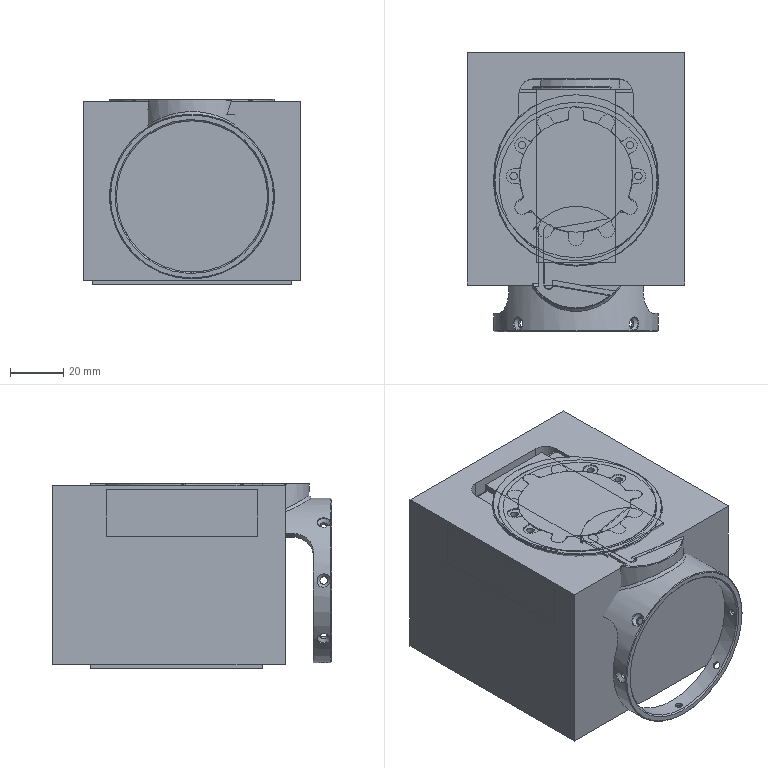NC program | NX | posted with a generic post | part box 82 x 105.2 x 70 mm
Lines 1 to 1140 of 2964:
N10 G17 G21 G94 G90
(外形动态铣_2 , TOOL : 粗刀D10)
N12 T15 M6
N14 G53
N16 G17 G0 G90 X-52.043 Y-12.093 B0. C0. S8500 M3
N18 G43 Z10. H15
N20 G94 G1 Z-1.42 F4500.
N22 Z-2.42
N24 X-50.413 Y-11.807
N26 G3 X-50.062 Y-11.562 R0.505
N28 X-49.643 Y-10.589 R3.413
N30 X-49.24 Y-8.159 R13.674
N32 X-49.052 Y-4.148 R57.416
N34 X-48.999 Y6.539 R617.695
N36 G1 X-48.995 Y30.289
N38 G2 X-48.67 Y32.126 R5.442
N40 X-47.193 Y34.11 R4.969
N42 X-44.793 Y35.433 R7.843
N44 X-41.628 Y36.142 R15.116
N46 X-37.264 Y36.43 R45.199
N48 X-28.39 Y36.499 R363.791
N50 G1 X42.61 Y36.498
N52 G2 X44.458 Y36.233 R5.973
N54 X46.495 Y34.832 R4.826
N56 X47.87 Y32.468 R7.551
N58 X48.602 Y29.434 R14.17
N60 X48.909 Y25.448 R38.306
N62 X48.997 Y17.949 R240.76
N64 G1 X48.995 Y-30.301
N66 G2 X48.668 Y-32.138 R5.474
N68 X47.277 Y-34.034 R4.92
N70 X45.018 Y-35.348 R7.552
N72 X41.866 Y-36.11 R14.168
N74 X37.629 Y-36.419 R41.423
N76 X29.755 Y-36.498 R283.099
N78 G1 X-42.745 Y-36.495
N80 G2 X-44.585 Y-36.186 R5.514
N82 X-46.579 Y-34.723 R4.919
N84 X-47.873 Y-32.444 R7.748
N86 X-48.621 Y-29.283 R14.522
N88 X-48.909 Y-25.42 R38.94
N90 X-48.998 Y-18.171 R233.446
N92 X-48.992 Y-14.546 R296.157
N94 X-48.757 Y-12.183 R24.037
N96 G3 X-48.103 Y-4.487 R64.834
N98 X-48.005 Y2.426 R246.922
N100 X-48. Y10.665 R1000.
N102 G1 X-47.999 Y27.917
N104 G2 X-46.344 Y32.109 R5.886
N106 X-43.67 Y33.95 R8.334
N108 X-40.441 Y34.904 R14.019
N110 X-36.342 Y35.342 R32.642
N112 X-30.219 Y35.486 R134.565
N114 X-24.094 Y35.499 R1000.
N116 G1 X40.416 Y35.498
N118 G2 X44.609 Y33.845 R5.88
N120 X46.45 Y31.17 R8.332
N122 X47.404 Y27.94 R14.057
N124 X47.842 Y23.841 R32.645
N126 X47.986 Y17.719 R134.554
N128 X47.999 Y11.594 R1000.
N130 G1 X47.998 Y-27.906
N132 G2 X46.348 Y-32.101 R5.882
N134 X43.671 Y-33.947 R8.336
N136 X40.442 Y-34.903 R14.049
N138 X36.343 Y-35.342 R32.586
N140 X30.22 Y-35.486 R134.246
N142 X23.97 Y-35.499 R1000.
N144 G1 X-40.416 Y-35.498
N146 G2 X-44.608 Y-33.841 R5.895
N148 X-46.447 Y-31.171 R8.316
N150 X-47.403 Y-27.941 R14.016
N152 X-47.842 Y-23.843 R32.589
N154 X-47.978 Y-16.22 R133.037
N156 X-47.763 Y-12.978 R44.65
N158 G3 X-47.291 Y-7.633 R159.7
N160 X-47.032 Y0.199 R149.4
N162 X-46.999 Y12.038 R1000.
N164 G1 X-46.996 Y25.913
N166 G2 X-46.54 Y28.484 R7.422
N168 X-44.24 Y31.56 R7.209
N170 X-41.152 Y33.205 R10.519
N172 X-37.375 Y34.05 R19.181
N174 X-32.64 Y34.399 R49.593
N176 X-25.141 Y34.496 R237.63
N178 G1 X38.359
N180 G2 X41.282 Y33.917 R7.449
N182 X44.32 Y31.392 R7.377
N184 X45.835 Y28.253 R11.074
N186 X46.602 Y24.458 R20.664
N188 X46.923 Y19.344 R57.679
N190 X46.998 Y9.97 R373.189
N192 G1 X46.995 Y-25.905
N194 G2 X46.446 Y-28.708 R7.345
N196 X44.241 Y-31.556 R7.239
N198 X41.153 Y-33.203 R10.504
N200 X37.378 Y-34.049 R19.152
N202 X32.643 Y-34.399 R49.518
N204 X25.144 Y-34.497 R234.014
N206 G1 X-38.356 Y-34.495
N208 G2 X-41.279 Y-33.916 R7.474
N210 X-44.32 Y-31.388 R7.386
N212 X-45.805 Y-28.35 R10.943
N214 X-46.603 Y-24.437 R20.53
N216 X-46.917 Y-19.573 R56.206
N218 X-46.738 Y-13.329 R55.96
N220 G3 X-46.333 Y-8.017 R338.621
N222 X-46.036 Y0.826 R173.15
N224 X-45.997 Y7.041 R606.66
N226 G1 X-45.995 Y23.915
N228 G2 X-45.649 Y26.509 R9.755
N230 X-43.262 Y30.146 R7.592
N232 X-40.135 Y31.967 R10.648
N234 X-36.264 Y32.943 R18.429
N236 X-31.285 Y33.372 R46.14
N238 X-24.161 Y33.493 R207.022
N240 G1 X35.839 Y33.498
N242 G2 X37.958 Y33.376 R13.815
N244 X42.673 Y30.725 R7.611
N246 X44.523 Y27.479 R10.701
N248 X45.466 Y23.6 R18.976
N250 X45.879 Y18.619 R48.048
N252 X45.994 Y11.12 R216.833
N254 G1 Y-23.88
N256 G2 X45.656 Y-26.474 R9.709
N258 X43.217 Y-30.181 R7.682
N260 X39.942 Y-32.038 R10.821
N262 X36.181 Y-32.955 R18.916
N264 X31.451 Y-33.364 R44.813
N266 X24.453 Y-33.492 R189.178
N268 G1 X19.453 Y-33.498
N270 X-36.422 Y-33.494
N272 G2 X-39.016 Y-33.145 R9.759
N274 X-42.642 Y-30.762 R7.606
N276 X-44.465 Y-27.636 R10.626
N278 X-45.461 Y-23.642 R18.622
N280 X-45.836 Y-16.285 R42.637
N282 X-45.592 Y-11.792 R107.085
N284 G3 X-45.034 Y1.823 R203.464
N286 X-44.999 Y14.288 R986.967
N288 G2 X-44.991 Y22.288 R944.802
N290 X-44.699 Y24.766 R11.344
N292 X-41.906 Y29.128 R8.152
N294 X-38.51 Y31.005 R11.434
N296 X-34.501 Y31.955 R20.428
N298 X-29.52 Y32.368 R50.119
N300 X-22.022 Y32.493 R213.614
N302 G1 X34.228 Y32.497
N304 G2 X36.595 Y32.333 R14.646
N306 X41.655 Y29.368 R8.135
N308 X43.47 Y26.094 R11.388
N310 X44.44 Y22.091 R20.004
N312 X44.865 Y17.111 R48.962
N314 X44.99 Y10.237 R197.067
N316 G1 X44.998 Y4.112
N318 X44.994 Y-22.013
N320 G2 X44.732 Y-24.619 R12.373
N322 X42.034 Y-29.016 R8.101
N324 X38.69 Y-30.935 R11.157
N326 X34.817 Y-31.908 R19.575
N328 X29.84 Y-32.355 R46.557
N330 X23.842 Y-32.483 R158.331
N332 X16.592 Y-32.498 R1000.
N334 G1 X-34.533 Y-32.494
N336 G2 X-37.018 Y-32.254 R12.688
N338 X-41.625 Y-29.404 R8.134
N340 X-43.503 Y-26.011 R11.403
N342 X-44.484 Y-21.753 R20.375
N344 X-44.75 Y-16.265 R38.136
N346 X-44.512 Y-10.895 R123.265
N348 G3 X-44.033 Y2.571 R242.716
N350 X-43.999 Y14.912 R1000.
N352 G2 X-43.988 Y20.662 R450.284
N354 X-43.674 Y23.389 R12.708
N356 X-40.889 Y27.883 R8.511
N358 X-37.744 Y29.75 R11.416
N360 X-33.893 Y30.804 R18.865
N362 X-29.297 Y31.296 R41.022
N364 X-22.925 Y31.476 R130.557
N366 X-16.175 Y31.497 R711.258
N368 G1 X-1.22 Y31.499
N370 G2 X0.49 Y31.58 R8.636
N372 G3 X8.042 Y31.498 R299.667
N374 G1 X32.791 Y31.493
N376 G2 X35.281 Y31.298 R15.428
N378 X40.466 Y28.285 R8.529
N380 X42.384 Y24.896 R11.816
N382 X43.403 Y20.778 R20.455
N384 X43.863 Y15.425 R50.095
N386 X43.992 Y7.927 R211.024
N388 G1 X43.998 Y-19.573
N390 G2 X43.885 Y-22.194 R22.421
N392 X42.721 Y-25.729 R8.758
N394 X40.142 Y-28.457 R8.995
N396 X36.654 Y-30.141 R12.821
N398 X32.376 Y-31.027 R23.489
N400 X26.891 Y-31.401 R60.265
N402 X17.642 Y-31.496 R327.657
N404 G1 X-32.733 Y-31.494
N406 G2 X-35.347 Y-31.288 R15.502
N408 X-40.677 Y-28.019 R8.552
N410 X-42.485 Y-24.611 R12.022
N412 X-43.427 Y-20.345 R19.892
N414 X-43.644 Y-15.228 R39.456
N416 X-43.495 Y-10.981 R124.985
N418 G3 X-43.013 Y5.432 R315.824
N420 X-42.997 Y14.911 R1000.
N422 G2 X-42.981 Y19.286 R191.99
N424 X-42.638 Y22.135 R13.374
N426 X-39.405 Y27.061 R8.879
N428 X-35.871 Y28.942 R12.502
N430 X-31.862 Y29.894 R21.869
N432 X-26.635 Y30.351 R50.776
N434 X-20.011 Y30.485 R179.698
N436 X-14.761 Y30.497 R672.427
N438 G1 X-4.209
N440 G3 X-3.912 Y30.561 R1.137
N442 G2 X-1.12 Y31.512 R7.843
N444 X0.49 Y31.58 R8.131
N446 X2.582 Y31.16 R8.072
N448 G3 X4.981 Y30.752 R13.63
N450 X9.227 Y30.55 R59.728
N452 X16.167 Y30.498 R370.195
N454 G1 X31.042 Y30.494
N456 G2 X33.783 Y30.308 R18.454
N458 X39.56 Y26.903 R8.9
N460 X41.441 Y23.371 R12.505
N462 X42.394 Y19.363 R21.879
N464 X42.85 Y14.135 R50.65
N466 X42.984 Y7.637 R175.115
N468 X42.997 Y1.262 R1000.
N470 G1 X42.994 Y-18.488
N472 G2 X42.818 Y-21.23 R19.428
N474 X39.406 Y-27.054 R8.9
N476 X35.874 Y-28.94 R12.483
N478 X31.867 Y-29.893 R21.838
N480 X26.889 Y-30.339 R49.303
N482 X19.266 Y-30.489 R192.116
N484 G1 X12.516 Y-30.497
N486 X-30.984 Y-30.494
N488 G2 X-33.726 Y-30.318 R19.375
N490 X-39.553 Y-26.905 R8.906
N492 X-41.47 Y-23.243 R12.262
N494 X-42.367 Y-18.842 R20.387
N496 X-42.54 Y-13.723 R44.569
N498 X-42.331 Y-7.705 R235.996
N500 G3 X-42.014 Y5.934 R343.25
N502 X-41.997 Y15.789 R1000.
N504 G2 X-41.931 Y18.787 R42.361
N506 X-41.367 Y21.725 R11.328
N508 X-38.221 Y26.019 R9.216
N510 X-34.669 Y27.9 R12.84
N512 X-30.417 Y28.9 R22.39
N514 X-25.314 Y29.342 R51.383
N516 X-18.815 Y29.483 R172.325
N518 X-12.316 Y29.497 R1000.
N520 G1 X-6.256 Y29.502
N522 G3 X-5.407 Y29.562 R5.192
N524 X-5.162 Y29.683 R0.915
N526 G2 X-3.842 Y30.603 R8.091
N528 G3 X-5.162 Y29.683 R8.091
N530 G1 X-5.312 Y29.552
N532 G2 X-6.213 Y29.163 R3.503
N534 X-8.39 Y28.771 R12.394
N536 X-12.363 Y28.557 R50.932
N538 X-20.564 Y28.459 R935.716
N540 G3 X-26.809 Y28.22 R106.277
N542 X-31.39 Y27.609 R34.478
N544 X-34.836 Y26.51 R16.633
N546 X-37.92 Y24.379 R10.048
N548 X-40.045 Y20.722 R9.193
N550 X-40.695 Y17.416 R16.745
N552 X-40.942 Y12.924 R55.167
N554 X-41.025 Y4.616 R726.109
N556 G2 X-41.396 Y-9.297 R393.877
N558 G3 X-41.503 Y-15.17 R101.056
N560 X-41.114 Y-19.774 R31.138
N562 X-40.033 Y-23.485 R15.483
N564 X-37.728 Y-26.717 R9.409
N566 X-34.477 Y-28.531 R9.01
N568 X-31.173 Y-29.191 R16.521
N570 X-26.681 Y-29.442 R53.722
N572 X-17.806 Y-29.497 R450.117
N574 G1 X17.694 Y-29.492
N576 G3 X25.442 Y-29.376 R230.25
N578 X30.675 Y-28.969 R55.007
N580 X34.58 Y-28.114 R22.016
N582 X37.816 Y-26.511 R11.851
N584 X40.914 Y-22.336 R8.62
N586 X41.633 Y-19.173 R15.009
N588 X41.919 Y-15.059 R42.907
N590 X41.996 Y-7.56 R267.03
N592 G1 X41.993 Y4.94
N594 G3 X41.88 Y12.814 R239.855
N596 X41.486 Y18.047 R56.79
N598 X40.693 Y21.835 R22.833
N600 X39.088 Y25.21 R12.149
N602 X34.836 Y28.414 R8.646
N604 X31.672 Y29.133 R14.996
N606 X27.559 Y29.419 R42.863
N608 X20.31 Y29.496 R260.08
N610 G2 X10.757 Y29.534 R713.841
N612 X5.951 Y29.733 R70.138
N614 G1 X5.269 Y29.802
N616 G2 X4.875 Y29.922 R0.945
N618 G3 X2.582 Y31.16 R8.052
N620 G2 X4.875 Y29.922 R8.052
N622 G1 X4.947 Y29.864
N624 X5.042 Y29.784
N626 G3 X6.286 Y29.249 R4.498
N628 X8.654 Y28.815 R14.157
N630 X12.871 Y28.569 R52.321
N632 X21.3 Y28.493 R399.736
N634 G2 X27.674 Y28.388 R169.322
N636 X31.405 Y28.04 R30.536
N638 X34.392 Y27.155 R11.547
N640 X38.033 Y23.982 R9.07
N642 X39.664 Y20.477 R13.232
N644 X40.51 Y16.317 R24.111
N646 X40.884 Y11.082 R59.052
N648 X40.994 Y2.208 R279.865
N650 G1 Y-8.167
N652 G2 X40.903 Y-14.791 R195.904
N654 X40.6 Y-18.527 R35.11
N656 X39.76 Y-21.656 R12.389
N658 X36.702 Y-25.38 R8.91
N660 X33.233 Y-27.082 R12.776
N662 X28.961 Y-27.992 R23.312
N664 X23.727 Y-28.379 R57.96
N666 X16.103 Y-28.492 R246.411
N668 G1 X-20.147 Y-28.494
N670 G2 X-27.146 Y-28.408 R218.621
N672 X-30.883 Y-28.118 R36.618
N674 X-33.789 Y-27.401 R12.993
N676 X-37.856 Y-24.183 R8.803
N678 X-39.574 Y-20.454 R12.348
N680 X-40.275 Y-16.396 R21.455
N682 X-40.409 Y-11.275 R51.249
N684 X-40.187 Y-3.623 R529.429
N686 G3 X-39.997 Y8.44 R510.163
N688 G2 X-39.87 Y14.313 R149.073
N690 X-39.475 Y18.039 R27.327
N692 X-38.382 Y21.218 R10.734
N694 X-35.243 Y24.56 R9.389
N696 X-31.589 Y26.199 R13.778
N698 X-27.298 Y27.031 R25.595
N700 X-21.687 Y27.4 R66.137
N702 X-14.387 Y27.525 R515.107
N704 G3 X-9.576 Y27.729 R70.901
N706 X-6.888 Y28.165 R15.367
N708 G1 X-6.696 Y28.221
N710 G3 X-6.339 Y28.431 R0.832
N712 G2 X-5.262 Y29.596 R7.302
N714 G3 X-6.339 Y28.431 R7.302
N716 G1 X-6.433 Y28.306
N718 G2 X-7.184 Y27.773 R2.687
N720 X-9.234 Y27.107 R8.402
N722 X-12.749 Y26.683 R25.968
N724 X-16.619 Y26.524 R102.043
N726 G3 X-22.735 Y26.342 R297.712
N728 X-27.712 Y25.89 R49.196
N730 X-31.592 Y24.945 R20.267
N732 X-34.66 Y23.28 R11.107
N734 X-37.374 Y19.746 R9.308
N736 X-38.422 Y16.154 R15.05
N738 X-38.859 Y11.804 R36.031
N740 X-39.006 Y6.306 R158.026
N742 G2 X-39.333 Y-8.196 R608.97
N744 G3 X-39.354 Y-13.945 R89.253
N746 X-38.885 Y-18.29 R27.31
N748 X-37.743 Y-21.719 R13.501
N750 X-33.706 Y-25.71 R8.788
N752 X-30.266 Y-26.834 R13.668
N754 X-26.047 Y-27.325 R31.498
N756 X-19.675 Y-27.483 R129.603
N758 X-13.05 Y-27.496 R1000.
N760 G1 X14.45 Y-27.494
N762 G3 X22.824 Y-27.391 R279.68
N764 X28.183 Y-27.008 R58.98
N766 X32.096 Y-26.197 R22.641
N768 X35.256 Y-24.708 R11.796
N770 X38.349 Y-20.967 R9.027
N772 X39.392 Y-17.505 R14.513
N774 X39.835 Y-13.407 R33.346
N776 X39.978 Y-7.909 R116.859
N778 X39.961 Y7.216 R997.403
N780 X39.709 Y13.71 R102.34
N782 X39.109 Y18.04 R32.026
N784 X37.901 Y21.58 R14.965
N786 X33.467 Y25.848 R9.04
N788 X30.005 Y26.892 R14.509
N790 X25.907 Y27.336 R33.327
N792 X20.784 Y27.478 R118.032
N794 G2 X13.907 Y27.559 R565.575
N796 X9.381 Y27.813 R55.889
N798 X6.785 Y28.282 R15.874
N800 X6.468 Y28.387 R2.208
N802 X6.247 Y28.555 R0.912
N804 G3 X4.951 Y29.86 R8.014
N806 G2 X6.247 Y28.555 R8.014
N808 G1 X6.322 Y28.454
N810 G3 X6.597 Y28.187 R1.436
N812 X7.884 Y27.535 R4.826
N814 X10.285 Y26.973 R13.264
N816 X14.185 Y26.634 R38.66
N818 X21.087 Y26.473 R249.764
N820 G2 X26.332 Y26.259 R84.596
N822 X30.159 Y25.678 R23.668
N824 X33.163 Y24.47 R10.916
N826 X36.368 Y21.197 R9.509
N828 X37.876 Y17.503 R14.272
N830 X38.586 Y13.444 R27.152
N832 X38.923 Y7.58 R73.097
N834 X38.995 Y-2.17 R426.104
N836 X38.92 Y-10.669 R317.057
N838 X38.61 Y-15.282 R49.572
N840 X37.873 Y-18.697 R17.46
N842 X35.519 Y-22.487 R9.324
N844 X32.276 Y-24.599 R10.882
N846 X28.201 Y-25.771 R18.355
N848 X23.232 Y-26.302 R41.663
N850 X16.11 Y-26.48 R153.795
N852 X8.61 Y-26.496 R1000.
N854 G1 X-17.015 Y-26.493
N856 G2 X-24.264 Y-26.379 R192.417
N858 X-28.618 Y-25.984 R37.38
N860 X-31.867 Y-25.099 R14.458
N862 X-36.1 Y-21.456 R8.953
N864 X-37.509 Y-18.113 R12.543
N866 X-38.17 Y-14.047 R22.318
N868 X-38.304 Y-9.051 R55.958
N870 X-38.158 Y-2.388 R350.261
N872 G3 X-37.998 Y6.584 R797.582
N874 G2 X-37.786 Y12.329 R104.491
N876 X-37.284 Y16.042 R26.614
N878 X-36.147 Y19.208 R11.929
N880 X-32.79 Y22.71 R9.522
N882 X-29.126 Y24.281 R14.008
N884 X-24.952 Y25.056 R26.656
N886 X-20.09 Y25.396 R66.882
N888 G3 X-14.848 Y25.591 R855.554
N890 X-10.625 Y25.967 R40.556
N892 X-8.07 Y26.597 R12.919
N894 X-7.352 Y26.921 R6.489
N896 X-7.131 Y27.143 R1.087
N898 G2 X-6.433 Y28.306 R7.698
N900 G3 X-7.131 Y27.143 R7.698
N902 G1 X-7.184 Y27.03
N904 G2 X-7.387 Y26.756 R1.076
N906 X-8.557 Y25.96 R4.256
N908 X-11.09 Y25.164 R10.883
N910 X-14.904 Y24.688 R31.437
N912 X-20.689 Y24.361 R311.284
N914 G3 X-25.416 Y23.915 R51.922
N916 X-29.299 Y22.98 R20.496
N918 X-32.565 Y21.175 R10.942
N920 X-35.148 Y17.798 R9.744
N922 X-36.284 Y14.233 R15.161
N924 X-36.82 Y9.768 R33.917
N926 X-37.021 Y4.272 R136.052
N928 G2 X-37.242 Y-5.716 R1000.
N930 G3 X-37.253 Y-11.465 R104.694
N932 X-36.829 Y-15.816 R30.052
N934 X-35.811 Y-19.155 R13.918
N936 X-31.634 Y-23.494 R9.067
N938 X-28.1 Y-24.717 R14.297
N940 X-24.015 Y-25.263 R29.924
N942 X-18.644 Y-25.461 R94.027
N944 X-9.769 Y-25.496 R649.854
N946 G1 X-6.564
N948 X-6.409 Y-25.503
N950 G3 X4.807 Y-25.851 R26.389
N952 G2 X8.398 Y-25.586 R35.668
N954 X12.82 Y-25.508 R191.97
N956 G3 X20.192 Y-25.405 R370.149
N958 X25.678 Y-25.044 R63.902
N960 X29.719 Y-24.24 R23.284
N962 X32.785 Y-22.851 R11.991
N964 X36.012 Y-19.203 R9.363
N966 X37.196 Y-15.784 R14.2
N968 X37.755 Y-11.7 R29.163
N970 X37.963 Y-6.08 R91.677
N972 X37.934 Y6.545 R452.132
N974 X37.614 Y12.534 R77.605
N976 X36.884 Y16.717 R26.284
N978 X35.426 Y20.158 R12.691
N980 X31.635 Y23.543 R9.358
N982 X28.085 Y24.739 R14.621
N984 X23.873 Y25.283 R31.352
N986 X19.628 Y25.471 R101.97
N988 G2 X14.127 Y25.664 R191.439
N990 X10.188 Y26.09 R33.36
N992 X7.834 Y26.744 R11.537
N994 G1 X7.475 Y26.906
N996 G2 X7.086 Y27.24 R0.808
N998 G3 X6.313 Y28.466 R7.803
N1000 G2 X7.086 Y27.24 R7.803
N1002 G1 X7.139 Y27.127
N1004 G3 X7.34 Y26.842 R1.216
N1006 X8.48 Y26.044 R4.123
N1008 X10.886 Y25.25 R10.52
N1010 X14.666 Y24.743 R28.669
N1012 X17.555 Y24.572 R88.293
N1014 G2 X22.786 Y24.322 R263.526
N1016 X27.001 Y23.802 R32.256
N1018 X30.096 Y22.833 R14.314
N1020 X34.249 Y19.164 R9.469
N1022 X35.784 Y15.608 R13.833
N1024 X36.562 Y11.435 R25.757
N1026 X36.899 Y6.197 R65.479
N1028 X36.918 Y-7.676 R295.505
N1030 X36.621 Y-12.416 R56.371
N1032 X35.9 Y-16.092 R20.698
N1034 X34.386 Y-19.23 R10.668
N1036 X31.001 Y-22.137 R9.977
N1038 X27.25 Y-23.508 R15.421
N1040 X22.803 Y-24.176 R31.371
N1042 X17.186 Y-24.44 R89.019
N1044 G1 X11.015 Y-24.536
N1046 G3 X9.356 Y-24.584 R49.777
N1048 G2 X4.807 Y-25.851 R26.402
N1050 G3 X9.356 Y-24.584 R26.402
N1052 G1 X9.561 Y-24.505
N1054 X10.14 Y-24.269
N1056 G2 X12.332 Y-23.805 R11.031
N1058 X15.575 Y-23.549 R43.826
N1060 G3 X20.795 Y-23.29 R349.758
N1062 X25.386 Y-22.753 R39.48
N1064 X29.09 Y-21.646 R16.653
N1066 X33.8 Y-17.284 R9.685
N1068 X35.146 Y-13.528 R14.648
N1070 X35.735 Y-9.322 R30.239
N1072 X35.96 Y-3.203 R94.425
N1074 X35.875 Y6.296 R212.734
N1076 X35.468 Y11.528 R53.713
N1078 X34.598 Y15.426 R20.973
N1080 X33.021 Y18.535 R11.344
N1082 X29.228 Y21.582 R9.94
N1084 X25.666 Y22.734 R15.774
N1086 X21.58 Y23.286 R34.464
N1088 X16.522 Y23.624 R262.203
N1090 G2 X12.283 Y24.079 R43.312
N1092 X10.158 Y24.563 R17.08
N1094 G1 X9.991 Y24.634
N1096 X9.88 Y24.68
N1098 X9.127 Y24.967
N1100 G2 X7.796 Y25.682 R6.244
N1102 X7.585 Y26. R0.814
N1104 G3 X7.115 Y27.179 R7.091
N1106 G2 X7.585 Y26. R7.091
N1108 G3 X7.712 Y25.615 R2.262
N1110 X8.063 Y25.332 R0.605
N1112 G2 X9.127 Y24.967 R19.055
N1114 G1 X9.88 Y24.68
N1116 X9.991 Y24.634
N1118 X10.854 Y24.265
N1120 X11.288 Y24.06
N1122 X11.797 Y23.816
N1124 G3 X13.976 Y23.142 R10.003
N1126 X16.651 Y22.749 R29.934
N1128 X21.065 Y22.324 R325.625
N1130 G2 X24.896 Y21.754 R34.136
N1132 X28.206 Y20.643 R14.523
N1134 X32.433 Y16.673 R9.803
N1136 X33.873 Y13.083 R14.526
N1138 X34.609 Y8.775 R27.967
N1140 X34.922 Y2.91 R75.207
N1142 X34.867 Y-6.339 R166.954
N1144 X34.481 Y-10.945 R44.774
N1146 X33.606 Y-14.588 R18.141
N1148 X31.49 Y-18.106 R10.131
N1150 X28.067 Y-20.5 R10.819
N1152 X24.371 Y-21.659 R17.202
N1154 X19.788 Y-22.262 R37.875
N1156 X15.054 Y-22.584 R852.107
N1158 G3 X13.273 Y-22.759 R36.387
N1160 G1 X13.119 Y-22.806
N1162 G2 X10.079 Y-24.294 R25.546
N1164 G3 X13.119 Y-22.806 R25.546
N1166 G1 X13.451 Y-22.618
N1168 X13.558 Y-22.553
N1170 G2 X15.174 Y-21.991 R7.234
N1172 X18.067 Y-21.511 R28.569
N1174 G3 X21.525 Y-21.071 R176.294
N1176 X25.429 Y-20.215 R24.858
N1178 X28.688 Y-18.646 R12.015
N1180 X31.801 Y-15.032 R10.
N1182 X33.097 Y-11.391 R15.052
N1184 X33.724 Y-6.939 R30.721
N1186 X33.934 Y-0.319 R90.674
N1188 X33.724 Y6.802 R97.712
N1190 X33.133 Y11.259 R32.87
N1192 X31.953 Y14.809 R15.191
N1194 X27.85 Y19.147 R9.868
N1196 X24.372 Y20.522 R14.619
N1198 X20.567 Y21.247 R31.634
N1200 G1 X16.595 Y21.756
N1202 G2 X14.95 Y22.024 R32.683
N1204 X14.711 Y22.123 R0.942
N1206 G3 X11.797 Y23.816 R25.542
N1208 G2 X14.711 Y22.123 R25.542
N1210 G1 X14.765 Y22.088
N1212 X15.177 Y21.802
N1214 G3 X16.792 Y21.136 R7.142
N1216 X18.955 Y20.622 R23.469
N1218 G2 X22.31 Y19.93 R119.03
N1220 X25.635 Y18.852 R18.258
N1222 X30.443 Y14.505 R10.174
N1224 X31.902 Y10.794 R14.799
N1226 X32.627 Y6.357 R28.81
N1228 X32.9 Y-0.135 R74.863
N1230 X32.689 Y-6.629 R76.174
N1232 X32.017 Y-10.948 R26.897
N1234 X30.691 Y-14.309 R13.035
N1236 X27.057 Y-17.914 R10.039
N1238 X23.366 Y-19.428 R15.143
N1240 X19.693 Y-20.197 R35.893
N1242 G3 X16.399 Y-20.78 R71.198
N1244 X16.003 Y-20.898 R1.511
N1246 G2 X13.555 Y-22.555 R25.771
N1248 G3 X16.003 Y-20.898 R25.771
N1250 G1 X16.273 Y-20.696
N1252 G2 X17.492 Y-20.065 R5.652
N1254 X19.212 Y-19.508 R18.314
N1256 G1 X19.395 Y-19.482
N1258 G3 X24.915 Y-18.102 R7.925
N1260 X27.229 Y-16.39 R17.
N1262 X30.216 Y-12.061 R11.763
N1264 X31.328 Y-7.968 R18.892
N1266 X31.795 Y-2.993 R40.791
N1268 X31.638 Y5.5 R70.402
N1270 X30.928 Y9.939 R27.692
N1272 X29.488 Y13.522 R13.581
N1274 X25.762 Y17.154 R10.317
N1276 X22.44 Y18.585 R16.516
N1278 X19.126 Y19.496 R58.633
N1280 G2 X17.707 Y19.89 R36.426
N1282 X17.459 Y20.01 R0.91
N1284 G3 X15.177 Y21.802 R26.197
N1286 G2 X17.459 Y20.01 R26.197
N1288 G1 X17.555 Y19.927
N1290 X17.77 Y19.73
N1292 G3 X19.016 Y18.978 R6.187
N1294 X20.962 Y18.159 R27.264
N1296 G2 X23.821 Y16.893 R28.733
N1298 X26.986 Y14.481 R11.478
N1300 X29.192 Y10.874 R11.892
N1302 X30.288 Y6.772 R19.43
N1304 X30.773 Y1.047 R41.832
N1306 X30.547 Y-5.57 R52.612
N1308 X29.752 Y-9.739 R22.921
N1310 X28.197 Y-13.137 R12.9
N1312 G1 X28.11 Y-13.305
N1314 G2 X24.915 Y-18.102 R7.975
N1316 G3 X28.11 Y-13.305 R7.975
N1318 G1 X28.142 Y-13.147
N1320 X28.183 Y-12.914
N1322 X28.247 Y-12.483
N1324 G2 X28.731 Y-10.036 R44.75
N1326 G3 X29.72 Y-0.855 R45.061
N1328 X29.413 Y5.132 R43.732
N1330 X28.489 Y9.272 R20.674
N1332 X26.442 Y12.97 R11.709
N1334 X23.606 Y15.425 R12.269
N1336 X20.976 Y16.879 R28.038
N1338 G2 X20.164 Y17.296 R13.333
N1340 G1 X20.05 Y17.39
N1342 G3 X17.77 Y19.73 R25.883
N1344 G2 X20.05 Y17.39 R25.883
N1346 G1 X20.098 Y17.333
N1348 X20.458 Y16.902
N1350 G3 X21.664 Y15.81 R10.731
N1352 G2 X23.569 Y14.228 R46.027
N1354 X27.292 Y8.672 R13.306
N1356 X28.303 Y4.423 R21.122
N1358 X28.588 Y-2.687 R39.942
N1360 X27.89 Y-8.769 R44.063
N1362 G3 X27.881 Y-9.07 R1.151
N1364 G2 X28.247 Y-12.483 R8.009
N1366 G3 X27.881 Y-9.07 R8.009
N1368 G1 X27.867 Y-9.025
N1370 X27.778 Y-8.791
N1372 G2 X27.565 Y-7.119 R7.752
N1374 X27.558 Y-5.124 R40.258
N1376 G3 X27.597 Y-0.891 R146.038
N1378 X27.465 Y2.356 R51.735
N1380 X26.668 Y6.904 R23.045
N1382 X23.359 Y12.618 R14.388
N1384 G1 X23.25 Y12.743
N1386 G3 X20.458 Y16.902 R25.942
N1388 G2 X23.25 Y12.743 R25.942
N1390 X26.434 Y0.914 R26.443
N1392 X26.544 Y-3.663 R73.468
N1394 G3 X26.621 Y-6.598 R37.415
N1396 X26.722 Y-6.86 R0.894
N1398 G2 X27.798 Y-8.843 R7.688
N1400 G3 X26.722 Y-6.86 R7.688
N1402 G1 X26.645 Y-6.762
N1404 G2 X26.371 Y-6.255 R2.056
N1406 X25.998 Y-4.911 R7.127
N1408 G1 X25.989 Y-4.736
N1410 G3 X26.434 Y0.914 R26.966
N1412 G2 X25.989 Y-4.736 R26.966
N1414 G1 X25.888 Y-5.226
N1416 G3 X25.908 Y-5.805 R2.033
N1418 X26.044 Y-6.064 R1.284
N1420 G1 X26.385 Y-6.43
N1422 X26.412 Y-6.463
N1424 X26.72 Y-6.857
N1426 X26.412 Y-6.463
N1428 X26.385 Y-6.43
N1430 X26.044 Y-6.064
N1432 G2 X25.838 Y-5.467 R0.637
N1434 G1 X25.889 Y-5.222
N1436 G2 X26.57 Y-4.862 R0.5
N1438 G1 X26.754 Y-4.938
N1440 X28.232 Y-5.551 Z-1.92
N1442 X29.164 Y-5.942 F15000.
N1444 G2 X29.366 Y-6.154 R0.528
N1446 G1 X29.758 Y-6.935
N1448 X30.121 Y-7.729
N1450 G2 X30.896 Y-11.534 R11.068
N1452 X30.326 Y-14.533 R8.563
N1454 G1 X28.834 Y-18.236
N1456 G2 X27.136 Y-20.246 R4.644
N1458 X26.169 Y-20.697 R4.165
N1460 G1 X21.881 Y-22.042
N1462 G2 X21.393 Y-21.854 R0.502
N1464 G1 X21.135 Y-21.516
N1466 X20.165 Y-20.244 Z-2.42 F4500.
N1468 X19.73 Y-19.674
N1470 G3 X19.395 Y-19.482 R0.5
N1472 G1 X19.063 Y-19.44
N1474 G3 X17.831 Y-19.483 R3.988
N1476 X17.574 Y-19.605 R0.896
N1478 G1 X17.321 Y-19.83
N1480 X16.907 Y-20.18
N1482 X16.273 Y-20.696
N1484 X16.907 Y-20.18
N1486 X17.321 Y-19.83
N1488 X17.574 Y-19.605
N1490 G2 X17.943 Y-19.314 R1.805
N1492 X18.337 Y-19.281 R0.599
N1494 G3 X19.063 Y-19.44 R7.328
N1496 G2 X19.473 Y-19.95 R0.5
N1498 G1 X19.467 Y-20.011 Z-2.401
N1500 X19.453 Y-20.071 Z-2.382
N1502 X18.873 Y-21.429 Z-1.92
N1504 X18.305 Y-22.742 F15000.
N1506 X18.228 Y-22.839
N1508 X18.131 Y-22.917
N1510 X16.846 Y-23.69
N1512 X15.552 Y-24.448
N1514 G2 X9.153 Y-27.234 R34.007
N1516 G1 X7.684 Y-27.703
N1518 X6.21 Y-28.151
N1520 G2 X1.229 Y-28.757 R17.453
N1522 G1 X-4.667 Y-28.616
N1524 G2 X-5.061 Y-28.307 R0.502
N1526 G1 X-5.263 Y-27.803
N1528 X-5.857 Y-26.318 Z-2.42 F4500.
N1530 X-6.063 Y-25.803
N1532 G3 X-6.409 Y-25.503 R0.5
N1534 G2 X-7.891 Y-25.085 R19.216
N1536 G3 X-10.319 Y-24.717 R15.212
N1538 X-14.358 Y-24.536 R68.46
N1540 G2 X-20.715 Y-24.403 R505.151
N1542 X-25.449 Y-24.045 R48.623
N1544 X-28.978 Y-23.242 R18.156
N1546 X-32.231 Y-21.379 R9.688
N1548 X-34.634 Y-18.064 R9.889
N1550 X-35.746 Y-14.361 R15.364
N1552 X-36.176 Y-9.886 R32.39
N1554 X-36.188 Y-4.136 R113.619
N1556 G1 X-36.024 Y3.976
N1558 G2 X-35.771 Y9.845 R105.887
N1560 X-35.183 Y13.924 R28.04
N1562 X-33.908 Y17.304 R12.477
N1564 X-30.48 Y20.785 R9.666
N1566 X-27.04 Y22.258 R14.071
N1568 X-22.871 Y23.062 R26.6
N1570 X-18.638 Y23.434 R78.602
N1572 G3 X-14.017 Y23.799 R107.676
N1574 X-10.618 Y24.387 R23.711
N1576 G1 X-10.472 Y24.427
N1578 X-9.887 Y24.678
N1580 X-9.024 Y25.006
N1582 X-8.906 Y25.048
N1584 G3 X-7.811 Y25.65 R5.612
N1586 X-7.595 Y25.968 R0.798
N1588 G2 X-7.168 Y27.064 R6.785
N1590 G3 X-7.595 Y25.968 R6.785
N1592 G2 X-7.737 Y25.574 R1.435
N1594 X-8.057 Y25.334 R0.598
N1596 G3 X-8.967 Y25.026 R17.716
N1598 G1 X-9.024 Y25.006
N1600 X-9.887 Y24.678
N1602 X-10.472 Y24.427
N1604 G3 X-12.023 Y23.703 R25.953
N1606 G2 X-14.412 Y23.022 R11.553
N1608 X-17.619 Y22.588 R39.418
N1610 G3 X-21.83 Y22.148 R216.833
N1612 X-25.881 Y21.387 R28.091
N1614 X-29.117 Y20.056 R13.477
N1616 X-32.843 Y16.111 R9.741
N1618 X-34.146 Y12.46 R14.909
N1620 X-34.757 Y8.257 R31.04
N1622 X-35.019 Y3.139 R94.942
N1624 X-35.202 Y-6.609 R370.374
N1626 X-35.014 Y-11.478 R54.048
N1628 X-34.329 Y-15.286 R20.381
N1630 X-32.86 Y-18.446 R10.777
N1632 X-29.682 Y-21.263 R9.32
N1634 X-26.055 Y-22.609 R14.132
N1636 X-21.978 Y-23.216 R28.782
N1638 X-17.61 Y-23.444 R78.743
N1640 G2 X-12.728 Y-23.602 R286.775
N1642 X-11.526 Y-23.68 R28.997
N1644 G1 X-11.384 Y-23.718
N1646 G3 X-7.798 Y-25.114 R25.731
N1648 G2 X-11.384 Y-23.718 R25.731
N1650 G1 X-11.614 Y-23.607
N1652 X-11.948 Y-23.437
N1654 G3 X-13.763 Y-22.93 R8.416
N1656 X-16.907 Y-22.572 R32.694
N1658 G2 X-21.243 Y-22.245 R235.275
N1660 X-25.071 Y-21.664 R28.857
N1662 X-28.463 Y-20.412 R13.214
N1664 X-32.136 Y-16.68 R9.383
N1666 X-33.47 Y-13.036 R13.801
N1668 X-34.013 Y-9.077 R26.344
N1670 X-34.143 Y-3.955 R71.651
N1672 X-33.892 Y5.791 R209.529
N1674 X-33.413 Y10.389 R41.836
N1676 X-32.419 Y13.997 R16.946
N1678 X-28.146 Y18.9 R9.935
N1680 X-24.574 Y20.372 R14.905
N1682 X-20.654 Y21.157 R31.751
N1684 X-16.732 Y21.683 R814.084
N1686 G3 X-14.972 Y21.985 R27.362
N1688 G1 X-14.827 Y22.045
N1690 G2 X-11.937 Y23.746 R26.478
N1692 G3 X-14.827 Y22.045 R26.478
N1694 G1 X-15.073 Y21.875
N1696 X-15.175 Y21.803
N1698 G2 X-16.55 Y21.174 R6.064
N1700 X-18.859 Y20.576 R20.717
N1702 G3 X-22.39 Y19.825 R142.102
N1704 X-25.825 Y18.687 R18.878
N1706 X-29.202 Y16.283 R10.373
N1708 X-31.377 Y12.727 R11.403
N1710 X-32.406 Y8.868 R19.172
N1712 X-32.908 Y4.021 R45.534
N1714 X-33.101 Y-6.1 R139.993
N1716 X-32.747 Y-10.708 R37.581
N1718 X-31.805 Y-14.329 R15.957
N1720 X-27.586 Y-19.147 R9.455
N1722 X-24.103 Y-20.513 R14.194
N1724 X-20.291 Y-21.191 R29.471
N1726 X-16.407 Y-21.608 R465.344
N1728 G2 X-14.784 Y-21.834 R31.207
N1730 G1 X-14.603 Y-21.894
N1732 G3 X-11.923 Y-23.449 R25.258
N1734 G2 X-14.603 Y-21.894 R25.258
N1736 G1 X-15.016 Y-21.613
N1738 G3 X-16.693 Y-20.974 R7.658
N1740 X-19.127 Y-20.456 R29.945
N1742 G2 X-22.316 Y-19.832 R63.145
N1744 X-25.514 Y-18.771 R16.463
N1746 X-28.379 Y-16.794 R9.645
N1748 X-30.56 Y-13.47 R10.501
N1750 X-31.622 Y-9.617 R16.919
N1752 X-32.035 Y-4.763 R37.143
N1754 X-31.8 Y4.98 R97.288
N1756 X-31.182 Y9.308 R31.46
N1758 X-29.939 Y12.836 R14.62
N1760 X-26.176 Y16.849 R10.27
N1762 X-22.871 Y18.368 R15.895
N1764 X-20.474 Y19.08 R35.988
N1766 G3 X-17.724 Y19.838 R66.684
N1768 G1 X-17.564 Y19.919
N1770 G2 X-15.098 Y21.858 R26.549
N1772 G3 X-17.564 Y19.919 R26.549
N1774 G1 X-17.666 Y19.827
N1776 X-17.849 Y19.657
N1778 G2 X-19.24 Y18.828 R6.751
N1780 X-21.685 Y17.801 R53.321
N1782 G3 X-24.509 Y16.452 R21.181
N1784 X-28.879 Y11.747 R10.883
N1786 X-30.194 Y7.832 R16.618
N1788 X-30.836 Y3.002 R35.798
N1790 X-30.945 Y-5.617 R72.402
N1792 X-30.396 Y-9.952 R26.926
N1794 X-29.284 Y-13.129 R13.06
N1796 X-26.965 Y-16.055 R9.384
N1798 G1 X-26.85 Y-16.161
N1800 G3 X-20.562 Y-19.539 R7.924
N1802 G2 X-17.189 Y-20.007 R17.816
N1804 G1 X-17.022 Y-20.084
N1806 G3 X-14.968 Y-21.645 R23.282
N1808 G2 X-17.022 Y-20.084 R23.282
N1810 G1 X-17.231 Y-19.91
N1812 G3 X-18.286 Y-19.355 R4.018
N1814 X-18.57 Y-19.338 R0.894
N1816 G2 X-20.627 Y-19.538 R7.734
N1818 G3 X-18.57 Y-19.338 R7.734
N1820 G2 X-18.179 Y-19.262 R1.842
N1822 X-17.781 Y-19.42 R0.595
N1824 G1 X-17.231 Y-19.91
N1826 G3 X-17.848 Y-19.368 R83.947
N1828 X-18.352 Y-19.283 R0.59
N1830 G2 X-25.442 Y-17.694 R7.907
N1832 X-26.85 Y-16.161 R7.723
N1834 X-27.854 Y-14.213 R7.891
N1836 X-29.159 Y-10.165 R27.745
N1838 X-29.866 Y-4.969 R31.62
N1840 X-29.637 Y4.393 R57.204
N1842 X-28.852 Y8.437 R24.049
N1844 X-27.247 Y11.948 R12.695
N1846 X-24.146 Y15.027 R11.646
N1848 X-21.33 Y16.65 R24.289
N1850 G1 X-20.33 Y17.156
N1852 G3 X-20.113 Y17.315 R0.922
N1854 G2 X-17.823 Y19.681 R25.942
N1856 G3 X-20.113 Y17.315 R25.942
N1858 G1 X-20.459 Y16.9
N1860 X-20.538 Y16.804
N1862 G2 X-21.783 Y15.684 R11.228
N1864 G3 X-23.623 Y14.169 R50.241
N1866 X-27.365 Y8.713 R13.336
N1868 X-28.432 Y4.479 R21.192
N1870 X-28.883 Y-2.25 R43.476
N1872 X-28.423 Y-8.1 R36.72
N1874 X-28.107 Y-9.694 R32.499
N1876 G1 X-28.104 Y-9.865
N1878 G3 X-27.854 Y-14.213 R7.986
N1880 G2 X-28.104 Y-9.865 R7.986
N1882 G1 X-28.036 Y-9.588
N1884 X-28.002 Y-9.468
N1886 G3 X-27.836 Y-7.629 R10.553
N1888 X-27.859 Y-4.245 R123.91
N1890 G2 X-27.659 Y1.874 R59.206
N1892 X-26.93 Y6.183 R26.656
N1894 X-26.28 Y8.205 R17.185
N1896 X-23.388 Y12.595 R14.349
N1898 G1 X-23.254 Y12.737
N1900 G2 X-20.533 Y16.811 R25.872
N1902 G3 X-23.254 Y12.737 R25.872
N1904 X-25.431 Y7.392 R26.221
N1906 X-26.605 Y1.138 R30.805
N1908 X-26.814 Y-4.106 R62.447
N1910 G2 X-26.862 Y-6.924 R58.941
N1912 X-26.954 Y-7.189 R0.903
N1914 G3 X-28.034 Y-9.578 R7.949
N1916 G2 X-26.954 Y-7.189 R7.949
N1918 G1 X-26.81 Y-6.984
N1920 G3 X-26.436 Y-6.017 R4.249
N1922 X-26.096 Y-4.101 R11.648
N1924 G2 X-25.431 Y7.392 R26.365
N1926 G3 X-26.096 Y-4.101 R26.365
N1928 G1 X-26.068 Y-4.275
N1930 X-25.995 Y-4.709
N1932 X-25.969 Y-4.831
N1934 G2 X-25.965 Y-5.852 R3.422
N1936 X-26.093 Y-6.116 R1.163
N1938 G3 X-26.811 Y-6.985 R7.275
N1940 G2 X-26.093 Y-6.116 R7.275
N1942 G3 X-25.849 Y-5.763 R0.845
N1944 X-25.84 Y-5.455 R0.648
N1946 G1 X-25.992 Y-4.721
N1948 G3 X-26.599 Y-4.33 R0.505
N1950 G1 X-28.029 Y-4.656
N1952 Z-1.42
N1954 G0 Z10.
(轮廓开粗_4 , TOOL : 粗刀D10)
N1956 X2. Y-43.85 S7500
N1958 Z-3.438
N1960 G1 Z-5.438 F4000.
N1962 G41 Y-38.65 D15
N1964 G3 X0. Y-36.65 R2.
N1966 G1 X-40.
N1968 G2 X-43.642 Y-35.142 R5.15
N1970 G1 X-44.642 Y-34.142
N1972 G2 X-46.15 Y-30.5 R5.15
N1974 G1 Y26.5
N1976 G2 X-44.642 Y30.142 R5.15
N1978 G1 X-39.642 Y35.142
N1980 G2 X-36. Y36.65 R5.15
N1982 G1 X36.
N1984 G2 X39.642 Y35.142 R5.15
N1986 G1 X44.642 Y30.142
N1988 G2 X46.15 Y26.5 R5.15
N1990 G1 Y-30.5
N1992 G2 X44.642 Y-34.142 R5.15
N1994 G1 X43.642 Y-35.142
N1996 G2 X40. Y-36.65 R5.15
N1998 G1 X0.
N2000 G3 X-2. Y-38.65 R2.
N2002 G1 Y-43.65
N2004 G40
N2006 Y-43.85
N2008 Z-3.438
N2010 G0 X2. Z-6.377
N2012 G1 Z-8.377
N2014 G41 Y-38.65
N2016 G3 X0. Y-36.65 R2.
N2018 G1 X-40.
N2020 G2 X-43.642 Y-35.142 R5.15
N2022 G1 X-44.642 Y-34.142
N2024 G2 X-46.15 Y-30.5 R5.15
N2026 G1 Y26.5
N2028 G2 X-44.642 Y30.142 R5.15
N2030 G1 X-39.642 Y35.142
N2032 G2 X-36. Y36.65 R5.15
N2034 G1 X36.
N2036 G2 X39.642 Y35.142 R5.15
N2038 G1 X44.642 Y30.142
N2040 G2 X46.15 Y26.5 R5.15
N2042 G1 Y-30.5
N2044 G2 X44.642 Y-34.142 R5.15
N2046 G1 X43.642 Y-35.142
N2048 G2 X40. Y-36.65 R5.15
N2050 G1 X0.
N2052 G3 X-2. Y-38.65 R2.
N2054 G1 Y-43.65
N2056 G40
N2058 Y-43.85
N2060 Z-6.377
N2062 G0 X2. Z-9.315
N2064 G1 Z-11.315
N2066 G41 Y-38.65
N2068 G3 X0. Y-36.65 R2.
N2070 G1 X-40.
N2072 G2 X-43.642 Y-35.142 R5.15
N2074 G1 X-44.642 Y-34.142
N2076 G2 X-46.15 Y-30.5 R5.15
N2078 G1 Y26.5
N2080 G2 X-44.642 Y30.142 R5.15
N2082 G1 X-39.642 Y35.142
N2084 G2 X-36. Y36.65 R5.15
N2086 G1 X36.
N2088 G2 X39.642 Y35.142 R5.15
N2090 G1 X44.642 Y30.142
N2092 G2 X46.15 Y26.5 R5.15
N2094 G1 Y-30.5
N2096 G2 X44.642 Y-34.142 R5.15
N2098 G1 X43.642 Y-35.142
N2100 G2 X40. Y-36.65 R5.15
N2102 G1 X0.
N2104 G3 X-2. Y-38.65 R2.
N2106 G1 Y-43.65
N2108 G40
N2110 Y-43.85
N2112 Z-9.315
N2114 G0 X2. Z-12.253
N2116 G1 Z-14.253
N2118 G41 Y-38.65
N2120 G3 X0. Y-36.65 R2.
N2122 G1 X-40.
N2124 G2 X-43.642 Y-35.142 R5.15
N2126 G1 X-44.642 Y-34.142
N2128 G2 X-46.15 Y-30.5 R5.15
N2130 G1 Y26.5
N2132 G2 X-44.642 Y30.142 R5.15
N2134 G1 X-39.642 Y35.142
N2136 G2 X-36. Y36.65 R5.15
N2138 G1 X36.
N2140 G2 X39.642 Y35.142 R5.15
N2142 G1 X44.642 Y30.142
N2144 G2 X46.15 Y26.5 R5.15
N2146 G1 Y-30.5
N2148 G2 X44.642 Y-34.142 R5.15
N2150 G1 X43.642 Y-35.142
N2152 G2 X40. Y-36.65 R5.15
N2154 G1 X0.
N2156 G3 X-2. Y-38.65 R2.
N2158 G1 Y-43.65
N2160 G40
N2162 Y-43.85
N2164 Z-12.253
N2166 G0 X2. Z-15.192
N2168 G1 Z-17.192
N2170 G41 Y-38.65
N2172 G3 X0. Y-36.65 R2.
N2174 G1 X-40.
N2176 G2 X-43.642 Y-35.142 R5.15
N2178 G1 X-44.642 Y-34.142
N2180 G2 X-46.15 Y-30.5 R5.15
N2182 G1 Y26.5
N2184 G2 X-44.642 Y30.142 R5.15
N2186 G1 X-39.642 Y35.142
N2188 G2 X-36. Y36.65 R5.15
N2190 G1 X36.
N2192 G2 X39.642 Y35.142 R5.15
N2194 G1 X44.642 Y30.142
N2196 G2 X46.15 Y26.5 R5.15
N2198 G1 Y-30.5
N2200 G2 X44.642 Y-34.142 R5.15
N2202 G1 X43.642 Y-35.142
N2204 G2 X40. Y-36.65 R5.15
N2206 G1 X0.
N2208 G3 X-2. Y-38.65 R2.
N2210 G1 Y-43.65
N2212 G40
N2214 Y-43.85
N2216 Z-15.192
N2218 G0 X2. Z-18.13
N2220 G1 Z-20.13
N2222 G41 Y-38.65
N2224 G3 X0. Y-36.65 R2.
N2226 G1 X-40.
N2228 G2 X-43.642 Y-35.142 R5.15
N2230 G1 X-44.642 Y-34.142
N2232 G2 X-46.15 Y-30.5 R5.15
N2234 G1 Y26.5
N2236 G2 X-44.642 Y30.142 R5.15
N2238 G1 X-39.642 Y35.142
N2240 G2 X-36. Y36.65 R5.15
N2242 G1 X36.
N2244 G2 X39.642 Y35.142 R5.15
N2246 G1 X44.642 Y30.142
N2248 G2 X46.15 Y26.5 R5.15
N2250 G1 Y-30.5
N2252 G2 X44.642 Y-34.142 R5.15
N2254 G1 X43.642 Y-35.142
N2256 G2 X40. Y-36.65 R5.15
N2258 G1 X0.
N2260 G3 X-2. Y-38.65 R2.
N2262 G1 Y-43.65
N2264 G40
N2266 Y-43.85
N2268 Z-18.13
N2270 G0 Z10.
N2272 M5